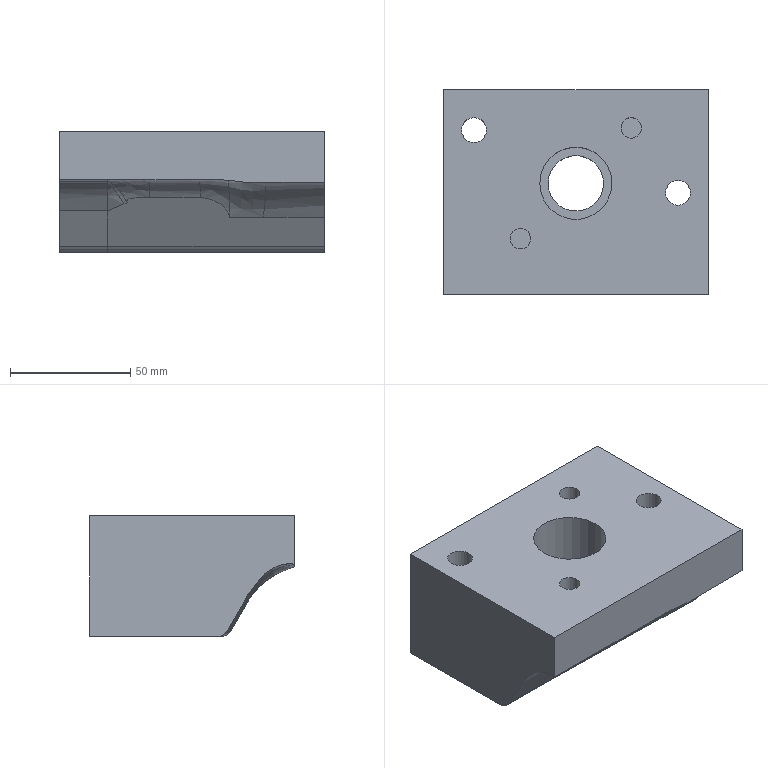Part | NX | features solid 2 | 1 solid | 34 faces | box 110 x 85 x 50.25 mm | volume 356395 mm3 | plane 14 | cylinder 10 | spline 10 | commonest cylinder face diameters 8.5 x2 10.3 x2 17 x2 30 x2 10 x1 23 x1